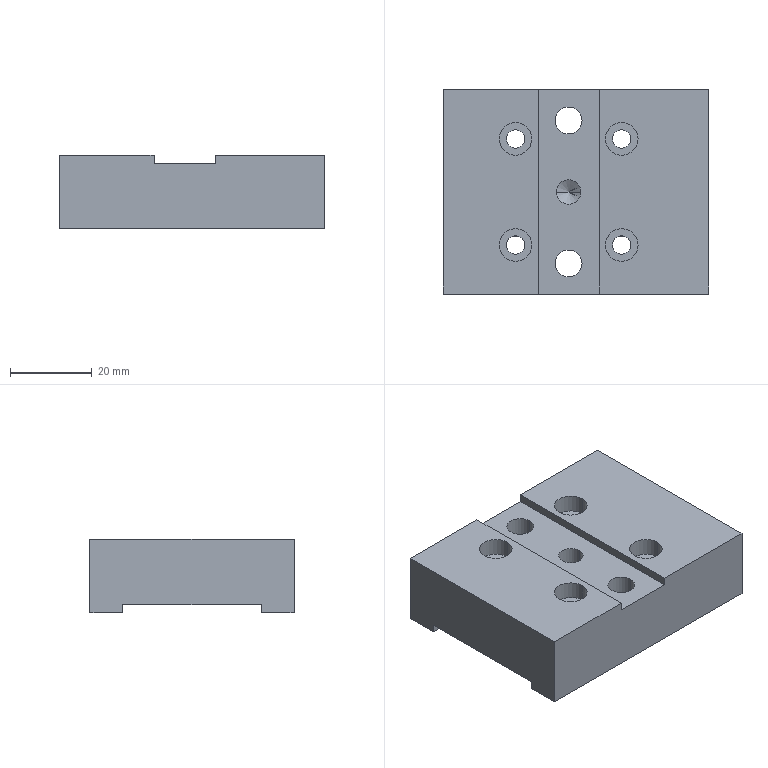Part | SolidWorks | features HoleWzd 6, Cut 3, Extrusion 1 | 1 solid | 66 faces | box 65 x 50 x 18 mm | volume 47739 mm3 | cylinder 34 | plane 22 | cone 10 | commonest cylinder face diameters 4.5 x8 8 x8 6 x6 5 x4 6.6 x4 11 x4